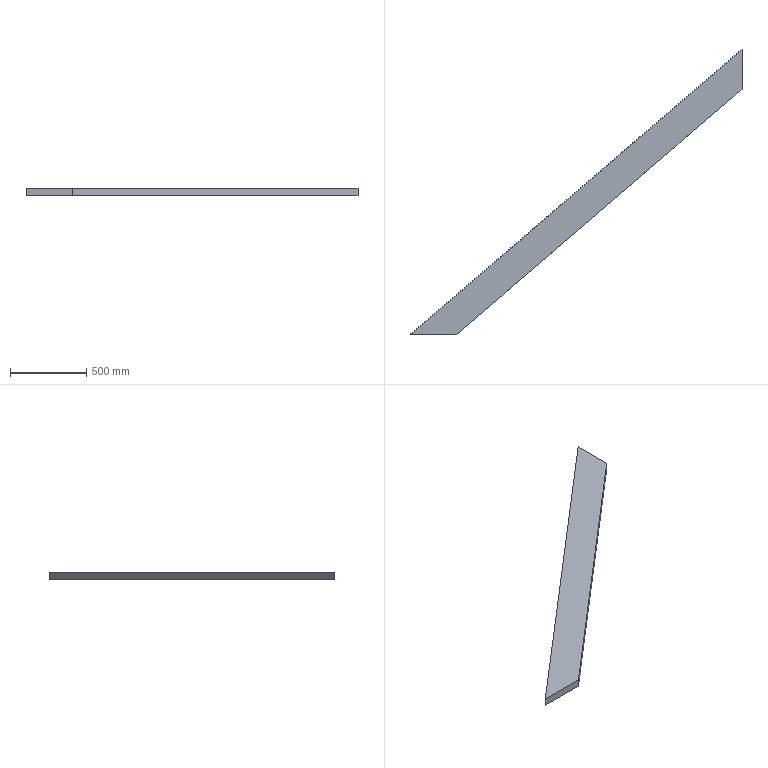Part | SolidWorks | features Extrusion 1 | 1 solid | 6 faces | box 2174 x 1869 x 50 mm | volume 26646819 mm3 | plane 6
STEP:
#1=CARTESIAN_POINT('',(960.482,14815.58,0.));
#2=VERTEX_POINT('',#1);
#3=CARTESIAN_POINT('',(-1213.383,12946.407,0.));
#4=VERTEX_POINT('',#3);
#5=CARTESIAN_POINT('',(960.482,14815.58,0.));
#6=DIRECTION('',(-0.7582,-0.652,0.));
#7=VECTOR('',#6,1000.);
#8=LINE('',#5,#7);
#9=EDGE_CURVE('',#2,#4,#8,.T.);
#10=ORIENTED_EDGE('',*,*,#9,.T.);
#11=CARTESIAN_POINT('',(-1213.383,12946.407,50.));
#12=VERTEX_POINT('',#11);
#13=CARTESIAN_POINT('',(-1213.383,12946.407,50.));
#14=DIRECTION('',(0.,0.,-1.));
#15=VECTOR('',#14,1000.);
#16=LINE('',#13,#15);
#17=EDGE_CURVE('',#12,#4,#16,.T.);
#18=ORIENTED_EDGE('',*,*,#17,.F.);
#19=CARTESIAN_POINT('',(960.482,14815.58,50.));
#20=VERTEX_POINT('',#19);
#21=CARTESIAN_POINT('',(960.482,14815.58,50.));
#22=DIRECTION('',(-0.7582,-0.652,0.));
#23=VECTOR('',#22,1000.);
#24=LINE('',#21,#23);
#25=EDGE_CURVE('',#20,#12,#24,.T.);
#26=ORIENTED_EDGE('',*,*,#25,.F.);
#27=CARTESIAN_POINT('',(960.482,14815.58,50.));
#28=DIRECTION('',(0.,0.,-1.));
#29=VECTOR('',#28,1000.);
#30=LINE('',#27,#29);
#31=EDGE_CURVE('',#20,#2,#30,.T.);
#32=ORIENTED_EDGE('',*,*,#31,.T.);
#33=EDGE_LOOP('',(#10,#18,#26,#32));
#34=FACE_OUTER_BOUND('',#33,.T.);
#35=CARTESIAN_POINT('',(960.482,14815.58,50.));
#36=DIRECTION('',(0.652,-0.7582,0.));
#37=DIRECTION('',(0.7582,0.652,0.));
#38=AXIS2_PLACEMENT_3D('',#35,#36,#37);
#39=PLANE('',#38);
#40=ADVANCED_FACE('',(#34),#39,.F.);
#41=CARTESIAN_POINT('',(-906.62,12946.407,0.));
#42=VERTEX_POINT('',#41);
#43=CARTESIAN_POINT('',(-1213.383,12946.407,0.));
#44=DIRECTION('',(1.,0.,0.));
#45=VECTOR('',#44,1000.);
#46=LINE('',#43,#45);
#47=EDGE_CURVE('',#4,#42,#46,.T.);
#48=ORIENTED_EDGE('',*,*,#47,.T.);
#49=CARTESIAN_POINT('',(-906.62,12946.407,50.));
#50=VERTEX_POINT('',#49);
#51=CARTESIAN_POINT('',(-906.62,12946.407,50.));
#52=DIRECTION('',(0.,0.,-1.));
#53=VECTOR('',#52,1000.);
#54=LINE('',#51,#53);
#55=EDGE_CURVE('',#50,#42,#54,.T.);
#56=ORIENTED_EDGE('',*,*,#55,.F.);
#57=CARTESIAN_POINT('',(-1213.383,12946.407,50.));
#58=DIRECTION('',(1.,0.,0.));
#59=VECTOR('',#58,1000.);
#60=LINE('',#57,#59);
#61=EDGE_CURVE('',#12,#50,#60,.T.);
#62=ORIENTED_EDGE('',*,*,#61,.F.);
#63=ORIENTED_EDGE('',*,*,#17,.T.);
#64=EDGE_LOOP('',(#48,#56,#62,#63));
#65=FACE_OUTER_BOUND('',#64,.T.);
#66=CARTESIAN_POINT('',(-1213.383,12946.407,50.));
#67=DIRECTION('',(0.,1.,0.));
#68=DIRECTION('',(0.,0.,1.));
#69=AXIS2_PLACEMENT_3D('',#66,#67,#68);
#70=PLANE('',#69);
#71=ADVANCED_FACE('',(#65),#70,.F.);
#72=CARTESIAN_POINT('',(960.482,14551.813,0.));
#73=VERTEX_POINT('',#72);
#74=CARTESIAN_POINT('',(-906.62,12946.407,0.));
#75=DIRECTION('',(0.7582,0.652,0.));
#76=VECTOR('',#75,1000.);
#77=LINE('',#74,#76);
#78=EDGE_CURVE('',#42,#73,#77,.T.);
#79=ORIENTED_EDGE('',*,*,#78,.T.);
#80=CARTESIAN_POINT('',(960.482,14551.813,50.));
#81=VERTEX_POINT('',#80);
#82=CARTESIAN_POINT('',(960.482,14551.813,50.));
#83=DIRECTION('',(0.,0.,-1.));
#84=VECTOR('',#83,1000.);
#85=LINE('',#82,#84);
#86=EDGE_CURVE('',#81,#73,#85,.T.);
#87=ORIENTED_EDGE('',*,*,#86,.F.);
#88=CARTESIAN_POINT('',(-906.62,12946.407,50.));
#89=DIRECTION('',(0.7582,0.652,0.));
#90=VECTOR('',#89,1000.);
#91=LINE('',#88,#90);
#92=EDGE_CURVE('',#50,#81,#91,.T.);
#93=ORIENTED_EDGE('',*,*,#92,.F.);
#94=ORIENTED_EDGE('',*,*,#55,.T.);
#95=EDGE_LOOP('',(#79,#87,#93,#94));
#96=FACE_OUTER_BOUND('',#95,.T.);
#97=CARTESIAN_POINT('',(-906.62,12946.407,50.));
#98=DIRECTION('',(-0.652,0.7582,0.));
#99=DIRECTION('',(-0.7582,-0.652,0.));
#100=AXIS2_PLACEMENT_3D('',#97,#98,#99);
#101=PLANE('',#100);
#102=ADVANCED_FACE('',(#96),#101,.F.);
#103=CARTESIAN_POINT('',(960.482,14551.813,0.));
#104=DIRECTION('',(0.,1.,0.));
#105=VECTOR('',#104,1000.);
#106=LINE('',#103,#105);
#107=EDGE_CURVE('',#73,#2,#106,.T.);
#108=ORIENTED_EDGE('',*,*,#107,.T.);
#109=ORIENTED_EDGE('',*,*,#31,.F.);
#110=CARTESIAN_POINT('',(960.482,14551.813,50.));
#111=DIRECTION('',(0.,1.,0.));
#112=VECTOR('',#111,1000.);
#113=LINE('',#110,#112);
#114=EDGE_CURVE('',#81,#20,#113,.T.);
#115=ORIENTED_EDGE('',*,*,#114,.F.);
#116=ORIENTED_EDGE('',*,*,#86,.T.);
#117=EDGE_LOOP('',(#108,#109,#115,#116));
#118=FACE_OUTER_BOUND('',#117,.T.);
#119=CARTESIAN_POINT('',(960.482,14551.813,50.));
#120=DIRECTION('',(-1.,0.,0.));
#121=DIRECTION('',(0.,0.,1.));
#122=AXIS2_PLACEMENT_3D('',#119,#120,#121);
#123=PLANE('',#122);
#124=ADVANCED_FACE('',(#118),#123,.F.);
#125=ORIENTED_EDGE('',*,*,#25,.T.);
#126=ORIENTED_EDGE('',*,*,#61,.T.);
#127=ORIENTED_EDGE('',*,*,#92,.T.);
#128=ORIENTED_EDGE('',*,*,#114,.T.);
#129=EDGE_LOOP('',(#125,#126,#127,#128));
#130=FACE_OUTER_BOUND('',#129,.T.);
#131=CARTESIAN_POINT('',(0.,0.,50.));
#132=DIRECTION('',(0.,0.,-1.));
#133=DIRECTION('',(-1.,0.,0.));
#134=AXIS2_PLACEMENT_3D('',#131,#132,#133);
#135=PLANE('',#134);
#136=ADVANCED_FACE('',(#130),#135,.F.);
#137=ORIENTED_EDGE('',*,*,#9,.F.);
#138=ORIENTED_EDGE('',*,*,#107,.F.);
#139=ORIENTED_EDGE('',*,*,#78,.F.);
#140=ORIENTED_EDGE('',*,*,#47,.F.);
#141=EDGE_LOOP('',(#137,#138,#139,#140));
#142=FACE_OUTER_BOUND('',#141,.T.);
#143=CARTESIAN_POINT('',(0.,0.,0.));
#144=DIRECTION('',(0.,0.,-1.));
#145=DIRECTION('',(-1.,0.,0.));
#146=AXIS2_PLACEMENT_3D('',#143,#144,#145);
#147=PLANE('',#146);
#148=ADVANCED_FACE('',(#142),#147,.T.);
#149=CLOSED_SHELL('',(#40,#71,#102,#124,#136,#148));
#150=MANIFOLD_SOLID_BREP('',#149);
#151=CARTESIAN_POINT('',(0.,0.,0.));
#152=DIRECTION('',(0.,0.,1.));
#153=DIRECTION('',(1.,0.,0.));
#154=AXIS2_PLACEMENT_3D('',#151,#152,#153);
#155=(LENGTH_UNIT()NAMED_UNIT(*)SI_UNIT(.MILLI.,.METRE.));
#156=UNCERTAINTY_MEASURE_WITH_UNIT(LENGTH_MEASURE(0.00001),#155,'','');
#157=(NAMED_UNIT(*)PLANE_ANGLE_UNIT()SI_UNIT($,.RADIAN.));
#158=(NAMED_UNIT(*)SI_UNIT($,.STERADIAN.)SOLID_ANGLE_UNIT());
#159=(GEOMETRIC_REPRESENTATION_CONTEXT(3)GLOBAL_UNCERTAINTY_ASSIGNED_CONTEXT((#156))GLOBAL_UNIT_ASSIGNED_CONTEXT((#155,#157,#158))REPRESENTATION_CONTEXT('',''));
#160=ADVANCED_BREP_SHAPE_REPRESENTATION('',(#150,#154),#159);